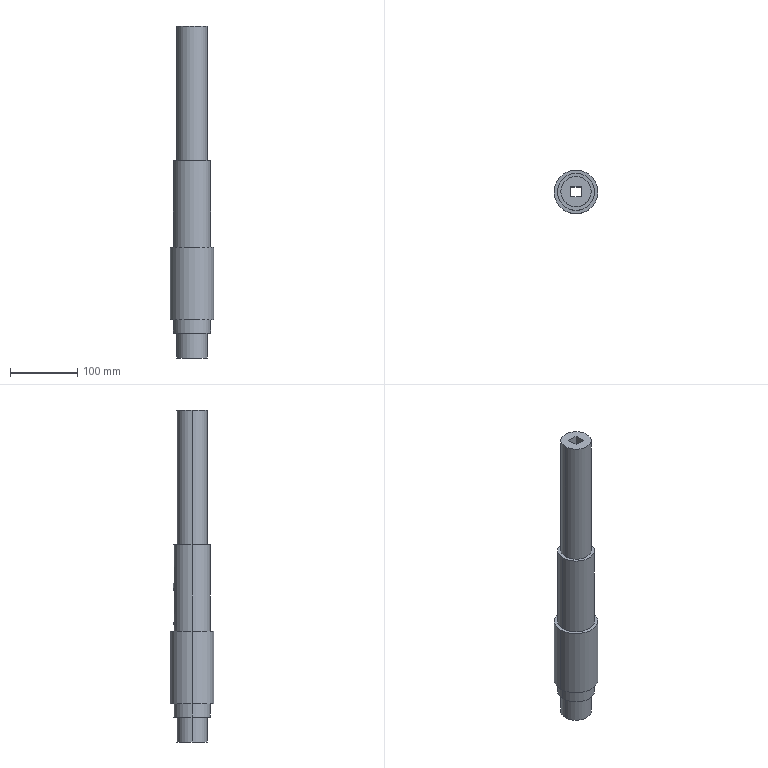Part | SolidWorks | features ICE 2, Chamfer 1, Revolution 1 | 1 solid | 29 faces | box 65 x 65 x 493 mm | volume 970539 mm3 | plane 17 | cylinder 12 | commonest cylinder face diameters 45 x4 55 x4 16 x2 65 x2
STEP:
#1=CARTESIAN_POINT('',(-22.5,0.,293.));
#2=VERTEX_POINT('',#1);
#3=CARTESIAN_POINT('',(22.5,0.,293.));
#4=VERTEX_POINT('',#3);
#5=CARTESIAN_POINT('',(0.,0.,293.));
#6=DIRECTION('',(0.,0.,-1.));
#7=DIRECTION('',(-1.,0.,0.));
#8=AXIS2_PLACEMENT_3D('',#5,#6,#7);
#9=CIRCLE('',#8,22.5);
#10=EDGE_CURVE('',#2,#4,#9,.T.);
#11=ORIENTED_EDGE('',*,*,#10,.T.);
#12=CARTESIAN_POINT('',(22.5,0.,93.));
#13=VERTEX_POINT('',#12);
#14=CARTESIAN_POINT('',(22.5,0.,0.));
#15=DIRECTION('',(0.,0.,-1.));
#16=VECTOR('',#15,1000.);
#17=LINE('',#14,#16);
#18=EDGE_CURVE('',#4,#13,#17,.T.);
#19=ORIENTED_EDGE('',*,*,#18,.T.);
#20=CARTESIAN_POINT('',(-22.5,0.,93.));
#21=VERTEX_POINT('',#20);
#22=CARTESIAN_POINT('',(0.,0.,93.));
#23=DIRECTION('',(0.,0.,-1.));
#24=DIRECTION('',(-1.,0.,0.));
#25=AXIS2_PLACEMENT_3D('',#22,#23,#24);
#26=CIRCLE('',#25,22.5);
#27=EDGE_CURVE('',#21,#13,#26,.T.);
#28=ORIENTED_EDGE('',*,*,#27,.F.);
#29=CARTESIAN_POINT('',(-22.5,0.,0.));
#30=DIRECTION('',(0.,0.,-1.));
#31=VECTOR('',#30,1000.);
#32=LINE('',#29,#31);
#33=EDGE_CURVE('',#2,#21,#32,.T.);
#34=ORIENTED_EDGE('',*,*,#33,.F.);
#35=EDGE_LOOP('',(#11,#19,#28,#34));
#36=FACE_OUTER_BOUND('',#35,.T.);
#37=CARTESIAN_POINT('',(0.,0.,0.));
#38=DIRECTION('',(0.,0.,-1.));
#39=DIRECTION('',(-1.,0.,0.));
#40=AXIS2_PLACEMENT_3D('',#37,#38,#39);
#41=CYLINDRICAL_SURFACE('',#40,22.5);
#42=ADVANCED_FACE('',(#36),#41,.T.);
#43=CARTESIAN_POINT('',(8.,26.311,-17.5));
#44=VERTEX_POINT('',#43);
#45=CARTESIAN_POINT('',(-8.,26.311,-17.5));
#46=VERTEX_POINT('',#45);
#47=CARTESIAN_POINT('',(8.,26.311,-17.5));
#48=CARTESIAN_POINT('',(8.,26.311,-18.032));
#49=CARTESIAN_POINT('',(7.948,26.327,-18.554));
#50=CARTESIAN_POINT('',(7.794,26.372,-19.323));
#51=CARTESIAN_POINT('',(7.73,26.391,-19.577));
#52=CARTESIAN_POINT('',(7.577,26.436,-20.081));
#53=CARTESIAN_POINT('',(7.487,26.461,-20.331));
#54=CARTESIAN_POINT('',(7.185,26.546,-21.056));
#55=CARTESIAN_POINT('',(6.94,26.612,-21.514));
#56=CARTESIAN_POINT('',(6.504,26.72,-22.165));
#57=CARTESIAN_POINT('',(6.347,26.758,-22.376));
#58=CARTESIAN_POINT('',(6.015,26.835,-22.781));
#59=CARTESIAN_POINT('',(5.841,26.873,-22.973));
#60=CARTESIAN_POINT('',(5.29,26.989,-23.523));
#61=CARTESIAN_POINT('',(4.89,27.065,-23.853));
#62=CARTESIAN_POINT('',(4.016,27.209,-24.439));
#63=CARTESIAN_POINT('',(3.556,27.273,-24.685));
#64=CARTESIAN_POINT('',(2.835,27.355,-24.985));
#65=CARTESIAN_POINT('',(2.589,27.379,-25.074));
#66=CARTESIAN_POINT('',(2.087,27.422,-25.227));
#67=CARTESIAN_POINT('',(1.829,27.44,-25.293));
#68=CARTESIAN_POINT('',(1.054,27.485,-25.448));
#69=CARTESIAN_POINT('',(0.5326,27.5,-25.499));
#70=CARTESIAN_POINT('',(-0.5171,27.5,-25.501));
#71=CARTESIAN_POINT('',(-1.05,27.485,-25.448));
#72=CARTESIAN_POINT('',(-2.079,27.426,-25.243));
#73=CARTESIAN_POINT('',(-2.579,27.383,-25.091));
#74=CARTESIAN_POINT('',(-3.308,27.301,-24.789));
#75=CARTESIAN_POINT('',(-3.547,27.271,-24.675));
#76=CARTESIAN_POINT('',(-4.008,27.207,-24.429));
#77=CARTESIAN_POINT('',(-4.231,27.173,-24.295));
#78=CARTESIAN_POINT('',(-4.663,27.103,-24.006));
#79=CARTESIAN_POINT('',(-4.871,27.066,-23.851));
#80=CARTESIAN_POINT('',(-5.275,26.99,-23.52));
#81=CARTESIAN_POINT('',(-5.47,26.951,-23.343));
#82=CARTESIAN_POINT('',(-6.024,26.835,-22.789));
#83=CARTESIAN_POINT('',(-6.354,26.758,-22.389));
#84=CARTESIAN_POINT('',(-6.933,26.613,-21.525));
#85=CARTESIAN_POINT('',(-7.185,26.546,-21.057));
#86=CARTESIAN_POINT('',(-7.586,26.434,-20.094));
#87=CARTESIAN_POINT('',(-7.739,26.389,-19.595));
#88=CARTESIAN_POINT('',(-7.895,26.343,-18.821));
#89=CARTESIAN_POINT('',(-7.934,26.331,-18.558));
#90=CARTESIAN_POINT('',(-7.987,26.315,-18.03));
#91=CARTESIAN_POINT('',(-8.,26.311,-17.766));
#92=CARTESIAN_POINT('',(-8.,26.311,-17.5));
#93=B_SPLINE_CURVE_WITH_KNOTS('',3,(#47,#48,#49,#50,#51,#52,#53,#54,#55,#56,#57,#58,#59,#60,#61,#62,#63,#64,#65,#66,#67,#68,#69,#70,#71,#72,#73,#74,#75,#76,#77,#78,#79,#80,#81,#82,#83,#84,#85,#86,#87,#88,#89,#90,#91,#92),.UNSPECIFIED.,.F.,.F.,(4,2,2,2,2,2,2,2,2,2,2,2,2,2,2,2,2,2,2,2,2,2,4),(0.,0.001571,0.002357,0.003142,0.004714,0.005499,0.006285,0.007856,0.009427,0.01021,0.011,0.01257,0.01414,0.01571,0.0165,0.01728,0.01807,0.01885,0.02043,0.022,0.02357,0.02435,0.02514),.UNSPECIFIED.);
#94=EDGE_CURVE('',#44,#46,#93,.T.);
#95=ORIENTED_EDGE('',*,*,#94,.F.);
#96=CARTESIAN_POINT('',(8.,26.311,19.5));
#97=VERTEX_POINT('',#96);
#98=CARTESIAN_POINT('',(8.,26.311,0.));
#99=DIRECTION('',(0.,0.,-1.));
#100=VECTOR('',#99,1000.);
#101=LINE('',#98,#100);
#102=EDGE_CURVE('',#97,#44,#101,.T.);
#103=ORIENTED_EDGE('',*,*,#102,.F.);
#104=CARTESIAN_POINT('',(-8.,26.311,19.5));
#105=VERTEX_POINT('',#104);
#106=CARTESIAN_POINT('',(-8.,26.311,19.5));
#107=CARTESIAN_POINT('',(-8.,26.311,20.032));
#108=CARTESIAN_POINT('',(-7.948,26.327,20.554));
#109=CARTESIAN_POINT('',(-7.794,26.372,21.323));
#110=CARTESIAN_POINT('',(-7.73,26.391,21.577));
#111=CARTESIAN_POINT('',(-7.577,26.436,22.081));
#112=CARTESIAN_POINT('',(-7.487,26.461,22.331));
#113=CARTESIAN_POINT('',(-7.185,26.546,23.056));
#114=CARTESIAN_POINT('',(-6.94,26.612,23.514));
#115=CARTESIAN_POINT('',(-6.504,26.72,24.165));
#116=CARTESIAN_POINT('',(-6.347,26.758,24.376));
#117=CARTESIAN_POINT('',(-6.015,26.835,24.781));
#118=CARTESIAN_POINT('',(-5.841,26.873,24.973));
#119=CARTESIAN_POINT('',(-5.29,26.989,25.523));
#120=CARTESIAN_POINT('',(-4.89,27.065,25.853));
#121=CARTESIAN_POINT('',(-4.016,27.209,26.439));
#122=CARTESIAN_POINT('',(-3.556,27.273,26.685));
#123=CARTESIAN_POINT('',(-2.835,27.355,26.985));
#124=CARTESIAN_POINT('',(-2.589,27.379,27.074));
#125=CARTESIAN_POINT('',(-2.087,27.422,27.227));
#126=CARTESIAN_POINT('',(-1.829,27.44,27.293));
#127=CARTESIAN_POINT('',(-1.054,27.485,27.448));
#128=CARTESIAN_POINT('',(-0.5326,27.5,27.499));
#129=CARTESIAN_POINT('',(0.5171,27.5,27.501));
#130=CARTESIAN_POINT('',(1.05,27.485,27.448));
#131=CARTESIAN_POINT('',(2.079,27.426,27.243));
#132=CARTESIAN_POINT('',(2.579,27.383,27.091));
#133=CARTESIAN_POINT('',(3.308,27.301,26.789));
#134=CARTESIAN_POINT('',(3.547,27.271,26.675));
#135=CARTESIAN_POINT('',(4.008,27.207,26.429));
#136=CARTESIAN_POINT('',(4.231,27.173,26.295));
#137=CARTESIAN_POINT('',(4.663,27.103,26.006));
#138=CARTESIAN_POINT('',(4.871,27.066,25.851));
#139=CARTESIAN_POINT('',(5.275,26.99,25.52));
#140=CARTESIAN_POINT('',(5.47,26.951,25.343));
#141=CARTESIAN_POINT('',(6.024,26.835,24.789));
#142=CARTESIAN_POINT('',(6.354,26.758,24.389));
#143=CARTESIAN_POINT('',(6.933,26.613,23.525));
#144=CARTESIAN_POINT('',(7.185,26.546,23.057));
#145=CARTESIAN_POINT('',(7.586,26.434,22.094));
#146=CARTESIAN_POINT('',(7.739,26.389,21.595));
#147=CARTESIAN_POINT('',(7.895,26.343,20.821));
#148=CARTESIAN_POINT('',(7.934,26.331,20.558));
#149=CARTESIAN_POINT('',(7.987,26.315,20.03));
#150=CARTESIAN_POINT('',(8.,26.311,19.766));
#151=CARTESIAN_POINT('',(8.,26.311,19.5));
#152=B_SPLINE_CURVE_WITH_KNOTS('',3,(#106,#107,#108,#109,#110,#111,#112,#113,#114,#115,#116,#117,#118,#119,#120,#121,#122,#123,#124,#125,#126,#127,#128,#129,#130,#131,#132,#133,#134,#135,#136,#137,#138,#139,#140,#141,#142,#143,#144,#145,#146,#147,#148,#149,#150,#151),.UNSPECIFIED.,.F.,.F.,(4,2,2,2,2,2,2,2,2,2,2,2,2,2,2,2,2,2,2,2,2,2,4),(0.,0.001571,0.002357,0.003142,0.004714,0.005499,0.006285,0.007856,0.009427,0.01021,0.011,0.01257,0.01414,0.01571,0.0165,0.01728,0.01807,0.01885,0.02043,0.022,0.02357,0.02435,0.02514),.UNSPECIFIED.);
#153=EDGE_CURVE('',#105,#97,#152,.T.);
#154=ORIENTED_EDGE('',*,*,#153,.F.);
#155=CARTESIAN_POINT('',(-8.,26.311,0.));
#156=DIRECTION('',(0.,0.,1.));
#157=VECTOR('',#156,1000.);
#158=LINE('',#155,#157);
#159=EDGE_CURVE('',#46,#105,#158,.T.);
#160=ORIENTED_EDGE('',*,*,#159,.F.);
#161=EDGE_LOOP('',(#95,#103,#154,#160));
#162=FACE_BOUND('',#161,.T.);
#163=CARTESIAN_POINT('',(-27.5,0.,93.));
#164=VERTEX_POINT('',#163);
#165=CARTESIAN_POINT('',(27.5,0.,93.));
#166=VERTEX_POINT('',#165);
#167=CARTESIAN_POINT('',(0.,0.,93.));
#168=DIRECTION('',(0.,0.,-1.));
#169=DIRECTION('',(-1.,0.,0.));
#170=AXIS2_PLACEMENT_3D('',#167,#168,#169);
#171=CIRCLE('',#170,27.5);
#172=EDGE_CURVE('',#164,#166,#171,.T.);
#173=ORIENTED_EDGE('',*,*,#172,.T.);
#174=CARTESIAN_POINT('',(27.5,0.,-35.5));
#175=VERTEX_POINT('',#174);
#176=CARTESIAN_POINT('',(27.5,0.,0.));
#177=DIRECTION('',(0.,0.,-1.));
#178=VECTOR('',#177,1000.);
#179=LINE('',#176,#178);
#180=EDGE_CURVE('',#166,#175,#179,.T.);
#181=ORIENTED_EDGE('',*,*,#180,.T.);
#182=CARTESIAN_POINT('',(-27.5,0.,-35.5));
#183=VERTEX_POINT('',#182);
#184=CARTESIAN_POINT('',(0.,0.,-35.5));
#185=DIRECTION('',(0.,0.,-1.));
#186=DIRECTION('',(-1.,0.,0.));
#187=AXIS2_PLACEMENT_3D('',#184,#185,#186);
#188=CIRCLE('',#187,27.5);
#189=EDGE_CURVE('',#183,#175,#188,.T.);
#190=ORIENTED_EDGE('',*,*,#189,.F.);
#191=CARTESIAN_POINT('',(-27.5,0.,0.));
#192=DIRECTION('',(0.,0.,-1.));
#193=VECTOR('',#192,1000.);
#194=LINE('',#191,#193);
#195=EDGE_CURVE('',#164,#183,#194,.T.);
#196=ORIENTED_EDGE('',*,*,#195,.F.);
#197=EDGE_LOOP('',(#173,#181,#190,#196));
#198=FACE_OUTER_BOUND('',#197,.T.);
#199=CARTESIAN_POINT('',(0.,0.,0.));
#200=DIRECTION('',(0.,0.,-1.));
#201=DIRECTION('',(-1.,0.,0.));
#202=AXIS2_PLACEMENT_3D('',#199,#200,#201);
#203=CYLINDRICAL_SURFACE('',#202,27.5);
#204=ADVANCED_FACE('',(#162,#198),#203,.T.);
#205=CARTESIAN_POINT('',(-32.5,0.,-35.5));
#206=VERTEX_POINT('',#205);
#207=CARTESIAN_POINT('',(32.5,0.,-35.5));
#208=VERTEX_POINT('',#207);
#209=CARTESIAN_POINT('',(0.,0.,-35.5));
#210=DIRECTION('',(0.,0.,-1.));
#211=DIRECTION('',(-1.,0.,0.));
#212=AXIS2_PLACEMENT_3D('',#209,#210,#211);
#213=CIRCLE('',#212,32.5);
#214=EDGE_CURVE('',#206,#208,#213,.T.);
#215=ORIENTED_EDGE('',*,*,#214,.T.);
#216=CARTESIAN_POINT('',(32.5,0.,-143.));
#217=VERTEX_POINT('',#216);
#218=CARTESIAN_POINT('',(32.5,0.,0.));
#219=DIRECTION('',(0.,0.,-1.));
#220=VECTOR('',#219,1000.);
#221=LINE('',#218,#220);
#222=EDGE_CURVE('',#208,#217,#221,.T.);
#223=ORIENTED_EDGE('',*,*,#222,.T.);
#224=CARTESIAN_POINT('',(-32.5,0.,-143.));
#225=VERTEX_POINT('',#224);
#226=CARTESIAN_POINT('',(0.,0.,-143.));
#227=DIRECTION('',(0.,0.,-1.));
#228=DIRECTION('',(-1.,0.,0.));
#229=AXIS2_PLACEMENT_3D('',#226,#227,#228);
#230=CIRCLE('',#229,32.5);
#231=EDGE_CURVE('',#225,#217,#230,.T.);
#232=ORIENTED_EDGE('',*,*,#231,.F.);
#233=CARTESIAN_POINT('',(-32.5,0.,0.));
#234=DIRECTION('',(0.,0.,-1.));
#235=VECTOR('',#234,1000.);
#236=LINE('',#233,#235);
#237=EDGE_CURVE('',#206,#225,#236,.T.);
#238=ORIENTED_EDGE('',*,*,#237,.F.);
#239=EDGE_LOOP('',(#215,#223,#232,#238));
#240=FACE_OUTER_BOUND('',#239,.T.);
#241=CARTESIAN_POINT('',(0.,0.,0.));
#242=DIRECTION('',(0.,0.,-1.));
#243=DIRECTION('',(-1.,0.,0.));
#244=AXIS2_PLACEMENT_3D('',#241,#242,#243);
#245=CYLINDRICAL_SURFACE('',#244,32.5);
#246=ADVANCED_FACE('',(#240),#245,.T.);
#247=CARTESIAN_POINT('',(-27.5,0.,-143.));
#248=VERTEX_POINT('',#247);
#249=CARTESIAN_POINT('',(27.5,0.,-143.));
#250=VERTEX_POINT('',#249);
#251=CARTESIAN_POINT('',(0.,0.,-143.));
#252=DIRECTION('',(0.,0.,-1.));
#253=DIRECTION('',(-1.,0.,0.));
#254=AXIS2_PLACEMENT_3D('',#251,#252,#253);
#255=CIRCLE('',#254,27.5);
#256=EDGE_CURVE('',#248,#250,#255,.T.);
#257=ORIENTED_EDGE('',*,*,#256,.T.);
#258=CARTESIAN_POINT('',(27.5,0.,-163.));
#259=VERTEX_POINT('',#258);
#260=CARTESIAN_POINT('',(27.5,0.,0.));
#261=DIRECTION('',(0.,0.,-1.));
#262=VECTOR('',#261,1000.);
#263=LINE('',#260,#262);
#264=EDGE_CURVE('',#250,#259,#263,.T.);
#265=ORIENTED_EDGE('',*,*,#264,.T.);
#266=CARTESIAN_POINT('',(-27.5,0.,-163.));
#267=VERTEX_POINT('',#266);
#268=CARTESIAN_POINT('',(0.,0.,-163.));
#269=DIRECTION('',(0.,0.,-1.));
#270=DIRECTION('',(-1.,0.,0.));
#271=AXIS2_PLACEMENT_3D('',#268,#269,#270);
#272=CIRCLE('',#271,27.5);
#273=EDGE_CURVE('',#267,#259,#272,.T.);
#274=ORIENTED_EDGE('',*,*,#273,.F.);
#275=CARTESIAN_POINT('',(-27.5,0.,0.));
#276=DIRECTION('',(0.,0.,-1.));
#277=VECTOR('',#276,1000.);
#278=LINE('',#275,#277);
#279=EDGE_CURVE('',#248,#267,#278,.T.);
#280=ORIENTED_EDGE('',*,*,#279,.F.);
#281=EDGE_LOOP('',(#257,#265,#274,#280));
#282=FACE_OUTER_BOUND('',#281,.T.);
#283=CARTESIAN_POINT('',(0.,0.,0.));
#284=DIRECTION('',(0.,0.,-1.));
#285=DIRECTION('',(-1.,0.,0.));
#286=AXIS2_PLACEMENT_3D('',#283,#284,#285);
#287=CYLINDRICAL_SURFACE('',#286,27.5);
#288=ADVANCED_FACE('',(#282),#287,.T.);
#289=CARTESIAN_POINT('',(-22.5,0.,-163.));
#290=VERTEX_POINT('',#289);
#291=CARTESIAN_POINT('',(22.5,0.,-163.));
#292=VERTEX_POINT('',#291);
#293=CARTESIAN_POINT('',(0.,0.,-163.));
#294=DIRECTION('',(0.,0.,-1.));
#295=DIRECTION('',(-1.,0.,0.));
#296=AXIS2_PLACEMENT_3D('',#293,#294,#295);
#297=CIRCLE('',#296,22.5);
#298=EDGE_CURVE('',#290,#292,#297,.T.);
#299=ORIENTED_EDGE('',*,*,#298,.T.);
#300=CARTESIAN_POINT('',(22.5,0.,-200.));
#301=VERTEX_POINT('',#300);
#302=CARTESIAN_POINT('',(22.5,0.,0.));
#303=DIRECTION('',(0.,0.,-1.));
#304=VECTOR('',#303,1000.);
#305=LINE('',#302,#304);
#306=EDGE_CURVE('',#292,#301,#305,.T.);
#307=ORIENTED_EDGE('',*,*,#306,.T.);
#308=CARTESIAN_POINT('',(-22.5,0.,-200.));
#309=VERTEX_POINT('',#308);
#310=CARTESIAN_POINT('',(0.,0.,-200.));
#311=DIRECTION('',(0.,0.,-1.));
#312=DIRECTION('',(-1.,0.,0.));
#313=AXIS2_PLACEMENT_3D('',#310,#311,#312);
#314=CIRCLE('',#313,22.5);
#315=EDGE_CURVE('',#309,#301,#314,.T.);
#316=ORIENTED_EDGE('',*,*,#315,.F.);
#317=CARTESIAN_POINT('',(-22.5,0.,0.));
#318=DIRECTION('',(0.,0.,-1.));
#319=VECTOR('',#318,1000.);
#320=LINE('',#317,#319);
#321=EDGE_CURVE('',#290,#309,#320,.T.);
#322=ORIENTED_EDGE('',*,*,#321,.F.);
#323=EDGE_LOOP('',(#299,#307,#316,#322));
#324=FACE_OUTER_BOUND('',#323,.T.);
#325=CARTESIAN_POINT('',(0.,0.,0.));
#326=DIRECTION('',(0.,0.,-1.));
#327=DIRECTION('',(-1.,0.,0.));
#328=AXIS2_PLACEMENT_3D('',#325,#326,#327);
#329=CYLINDRICAL_SURFACE('',#328,22.5);
#330=ADVANCED_FACE('',(#324),#329,.T.);
#331=CARTESIAN_POINT('',(-10.5,-10.5,-200.));
#332=VERTEX_POINT('',#331);
#333=CARTESIAN_POINT('',(10.5,-10.5,-200.));
#334=VERTEX_POINT('',#333);
#335=CARTESIAN_POINT('',(7.5,-10.5,-200.));
#336=DIRECTION('',(1.,0.,0.));
#337=VECTOR('',#336,1000.);
#338=LINE('',#335,#337);
#339=EDGE_CURVE('',#332,#334,#338,.T.);
#340=ORIENTED_EDGE('',*,*,#339,.T.);
#341=CARTESIAN_POINT('',(10.5,10.5,-200.));
#342=VERTEX_POINT('',#341);
#343=CARTESIAN_POINT('',(10.5,7.5,-200.));
#344=DIRECTION('',(0.,1.,0.));
#345=VECTOR('',#344,1000.);
#346=LINE('',#343,#345);
#347=EDGE_CURVE('',#334,#342,#346,.T.);
#348=ORIENTED_EDGE('',*,*,#347,.T.);
#349=CARTESIAN_POINT('',(-10.5,10.5,-200.));
#350=VERTEX_POINT('',#349);
#351=CARTESIAN_POINT('',(-7.5,10.5,-200.));
#352=DIRECTION('',(-1.,0.,0.));
#353=VECTOR('',#352,1000.);
#354=LINE('',#351,#353);
#355=EDGE_CURVE('',#342,#350,#354,.T.);
#356=ORIENTED_EDGE('',*,*,#355,.T.);
#357=CARTESIAN_POINT('',(-10.5,-7.5,-200.));
#358=DIRECTION('',(0.,-1.,0.));
#359=VECTOR('',#358,1000.);
#360=LINE('',#357,#359);
#361=EDGE_CURVE('',#350,#332,#360,.T.);
#362=ORIENTED_EDGE('',*,*,#361,.T.);
#363=EDGE_LOOP('',(#340,#348,#356,#362));
#364=FACE_BOUND('',#363,.T.);
#365=ORIENTED_EDGE('',*,*,#315,.T.);
#366=CARTESIAN_POINT('',(0.,0.,-200.));
#367=DIRECTION('',(0.,0.,-1.));
#368=DIRECTION('',(-1.,0.,0.));
#369=AXIS2_PLACEMENT_3D('',#366,#367,#368);
#370=CIRCLE('',#369,22.5);
#371=EDGE_CURVE('',#301,#309,#370,.T.);
#372=ORIENTED_EDGE('',*,*,#371,.T.);
#373=EDGE_LOOP('',(#365,#372));
#374=FACE_OUTER_BOUND('',#373,.T.);
#375=CARTESIAN_POINT('',(0.,0.,-200.));
#376=DIRECTION('',(0.,0.,-1.));
#377=DIRECTION('',(-1.,0.,0.));
#378=AXIS2_PLACEMENT_3D('',#375,#376,#377);
#379=PLANE('',#378);
#380=ADVANCED_FACE('',(#364,#374),#379,.T.);
#381=ORIENTED_EDGE('',*,*,#306,.F.);
#382=CARTESIAN_POINT('',(0.,0.,-163.));
#383=DIRECTION('',(0.,0.,-1.));
#384=DIRECTION('',(-1.,0.,0.));
#385=AXIS2_PLACEMENT_3D('',#382,#383,#384);
#386=CIRCLE('',#385,22.5);
#387=EDGE_CURVE('',#292,#290,#386,.T.);
#388=ORIENTED_EDGE('',*,*,#387,.T.);
#389=ORIENTED_EDGE('',*,*,#321,.T.);
#390=ORIENTED_EDGE('',*,*,#371,.F.);
#391=EDGE_LOOP('',(#381,#388,#389,#390));
#392=FACE_OUTER_BOUND('',#391,.T.);
#393=CARTESIAN_POINT('',(0.,0.,0.));
#394=DIRECTION('',(0.,0.,-1.));
#395=DIRECTION('',(-1.,0.,0.));
#396=AXIS2_PLACEMENT_3D('',#393,#394,#395);
#397=CYLINDRICAL_SURFACE('',#396,22.5);
#398=ADVANCED_FACE('',(#392),#397,.T.);
#399=ORIENTED_EDGE('',*,*,#273,.T.);
#400=CARTESIAN_POINT('',(0.,0.,-163.));
#401=DIRECTION('',(0.,0.,-1.));
#402=DIRECTION('',(-1.,0.,0.));
#403=AXIS2_PLACEMENT_3D('',#400,#401,#402);
#404=CIRCLE('',#403,27.5);
#405=EDGE_CURVE('',#259,#267,#404,.T.);
#406=ORIENTED_EDGE('',*,*,#405,.T.);
#407=EDGE_LOOP('',(#399,#406));
#408=FACE_OUTER_BOUND('',#407,.T.);
#409=ORIENTED_EDGE('',*,*,#298,.F.);
#410=ORIENTED_EDGE('',*,*,#387,.F.);
#411=EDGE_LOOP('',(#409,#410));
#412=FACE_BOUND('',#411,.T.);
#413=CARTESIAN_POINT('',(-22.5,0.,-163.));
#414=DIRECTION('',(0.,0.,-1.));
#415=DIRECTION('',(-1.,0.,0.));
#416=AXIS2_PLACEMENT_3D('',#413,#414,#415);
#417=PLANE('',#416);
#418=ADVANCED_FACE('',(#408,#412),#417,.T.);
#419=ORIENTED_EDGE('',*,*,#264,.F.);
#420=CARTESIAN_POINT('',(0.,0.,-143.));
#421=DIRECTION('',(0.,0.,-1.));
#422=DIRECTION('',(-1.,0.,0.));
#423=AXIS2_PLACEMENT_3D('',#420,#421,#422);
#424=CIRCLE('',#423,27.5);
#425=EDGE_CURVE('',#250,#248,#424,.T.);
#426=ORIENTED_EDGE('',*,*,#425,.T.);
#427=ORIENTED_EDGE('',*,*,#279,.T.);
#428=ORIENTED_EDGE('',*,*,#405,.F.);
#429=EDGE_LOOP('',(#419,#426,#427,#428));
#430=FACE_OUTER_BOUND('',#429,.T.);
#431=CARTESIAN_POINT('',(0.,0.,0.));
#432=DIRECTION('',(0.,0.,-1.));
#433=DIRECTION('',(-1.,0.,0.));
#434=AXIS2_PLACEMENT_3D('',#431,#432,#433);
#435=CYLINDRICAL_SURFACE('',#434,27.5);
#436=ADVANCED_FACE('',(#430),#435,.T.);
#437=ORIENTED_EDGE('',*,*,#231,.T.);
#438=CARTESIAN_POINT('',(0.,0.,-143.));
#439=DIRECTION('',(0.,0.,-1.));
#440=DIRECTION('',(-1.,0.,0.));
#441=AXIS2_PLACEMENT_3D('',#438,#439,#440);
#442=CIRCLE('',#441,32.5);
#443=EDGE_CURVE('',#217,#225,#442,.T.);
#444=ORIENTED_EDGE('',*,*,#443,.T.);
#445=EDGE_LOOP('',(#437,#444));
#446=FACE_OUTER_BOUND('',#445,.T.);
#447=ORIENTED_EDGE('',*,*,#256,.F.);
#448=ORIENTED_EDGE('',*,*,#425,.F.);
#449=EDGE_LOOP('',(#447,#448));
#450=FACE_BOUND('',#449,.T.);
#451=CARTESIAN_POINT('',(-32.5,0.,-143.));
#452=DIRECTION('',(0.,0.,-1.));
#453=DIRECTION('',(-1.,0.,0.));
#454=AXIS2_PLACEMENT_3D('',#451,#452,#453);
#455=PLANE('',#454);
#456=ADVANCED_FACE('',(#446,#450),#455,.T.);
#457=ORIENTED_EDGE('',*,*,#222,.F.);
#458=CARTESIAN_POINT('',(0.,0.,-35.5));
#459=DIRECTION('',(0.,0.,-1.));
#460=DIRECTION('',(-1.,0.,0.));
#461=AXIS2_PLACEMENT_3D('',#458,#459,#460);
#462=CIRCLE('',#461,32.5);
#463=EDGE_CURVE('',#208,#206,#462,.T.);
#464=ORIENTED_EDGE('',*,*,#463,.T.);
#465=ORIENTED_EDGE('',*,*,#237,.T.);
#466=ORIENTED_EDGE('',*,*,#443,.F.);
#467=EDGE_LOOP('',(#457,#464,#465,#466));
#468=FACE_OUTER_BOUND('',#467,.T.);
#469=CARTESIAN_POINT('',(0.,0.,0.));
#470=DIRECTION('',(0.,0.,-1.));
#471=DIRECTION('',(-1.,0.,0.));
#472=AXIS2_PLACEMENT_3D('',#469,#470,#471);
#473=CYLINDRICAL_SURFACE('',#472,32.5);
#474=ADVANCED_FACE('',(#468),#473,.T.);
#475=ORIENTED_EDGE('',*,*,#189,.T.);
#476=CARTESIAN_POINT('',(0.,0.,-35.5));
#477=DIRECTION('',(0.,0.,-1.));
#478=DIRECTION('',(-1.,0.,0.));
#479=AXIS2_PLACEMENT_3D('',#476,#477,#478);
#480=CIRCLE('',#479,27.5);
#481=EDGE_CURVE('',#175,#183,#480,.T.);
#482=ORIENTED_EDGE('',*,*,#481,.T.);
#483=EDGE_LOOP('',(#475,#482));
#484=FACE_BOUND('',#483,.T.);
#485=ORIENTED_EDGE('',*,*,#214,.F.);
#486=ORIENTED_EDGE('',*,*,#463,.F.);
#487=EDGE_LOOP('',(#485,#486));
#488=FACE_OUTER_BOUND('',#487,.T.);
#489=CARTESIAN_POINT('',(-27.5,0.,-35.5));
#490=DIRECTION('',(0.,0.,1.));
#491=DIRECTION('',(1.,0.,0.));
#492=AXIS2_PLACEMENT_3D('',#489,#490,#491);
#493=PLANE('',#492);
#494=ADVANCED_FACE('',(#484,#488),#493,.T.);
#495=ORIENTED_EDGE('',*,*,#180,.F.);
#496=CARTESIAN_POINT('',(0.,0.,93.));
#497=DIRECTION('',(0.,0.,-1.));
#498=DIRECTION('',(-1.,0.,0.));
#499=AXIS2_PLACEMENT_3D('',#496,#497,#498);
#500=CIRCLE('',#499,27.5);
#501=EDGE_CURVE('',#166,#164,#500,.T.);
#502=ORIENTED_EDGE('',*,*,#501,.T.);
#503=ORIENTED_EDGE('',*,*,#195,.T.);
#504=ORIENTED_EDGE('',*,*,#481,.F.);
#505=EDGE_LOOP('',(#495,#502,#503,#504));
#506=FACE_OUTER_BOUND('',#505,.T.);
#507=CARTESIAN_POINT('',(0.,0.,0.));
#508=DIRECTION('',(0.,0.,-1.));
#509=DIRECTION('',(-1.,0.,0.));
#510=AXIS2_PLACEMENT_3D('',#507,#508,#509);
#511=CYLINDRICAL_SURFACE('',#510,27.5);
#512=ADVANCED_FACE('',(#506),#511,.T.);
#513=ORIENTED_EDGE('',*,*,#27,.T.);
#514=CARTESIAN_POINT('',(0.,0.,93.));
#515=DIRECTION('',(0.,0.,-1.));
#516=DIRECTION('',(-1.,0.,0.));
#517=AXIS2_PLACEMENT_3D('',#514,#515,#516);
#518=CIRCLE('',#517,22.5);
#519=EDGE_CURVE('',#13,#21,#518,.T.);
#520=ORIENTED_EDGE('',*,*,#519,.T.);
#521=EDGE_LOOP('',(#513,#520));
#522=FACE_BOUND('',#521,.T.);
#523=ORIENTED_EDGE('',*,*,#172,.F.);
#524=ORIENTED_EDGE('',*,*,#501,.F.);
#525=EDGE_LOOP('',(#523,#524));
#526=FACE_OUTER_BOUND('',#525,.T.);
#527=CARTESIAN_POINT('',(-27.5,0.,93.));
#528=DIRECTION('',(0.,0.,1.));
#529=DIRECTION('',(1.,0.,0.));
#530=AXIS2_PLACEMENT_3D('',#527,#528,#529);
#531=PLANE('',#530);
#532=ADVANCED_FACE('',(#522,#526),#531,.T.);
#533=ORIENTED_EDGE('',*,*,#18,.F.);
#534=CARTESIAN_POINT('',(0.,0.,293.));
#535=DIRECTION('',(0.,0.,-1.));
#536=DIRECTION('',(-1.,0.,0.));
#537=AXIS2_PLACEMENT_3D('',#534,#535,#536);
#538=CIRCLE('',#537,22.5);
#539=EDGE_CURVE('',#4,#2,#538,.T.);
#540=ORIENTED_EDGE('',*,*,#539,.T.);
#541=ORIENTED_EDGE('',*,*,#33,.T.);
#542=ORIENTED_EDGE('',*,*,#519,.F.);
#543=EDGE_LOOP('',(#533,#540,#541,#542));
#544=FACE_OUTER_BOUND('',#543,.T.);
#545=CARTESIAN_POINT('',(0.,0.,0.));
#546=DIRECTION('',(0.,0.,-1.));
#547=DIRECTION('',(-1.,0.,0.));
#548=AXIS2_PLACEMENT_3D('',#545,#546,#547);
#549=CYLINDRICAL_SURFACE('',#548,22.5);
#550=ADVANCED_FACE('',(#544),#549,.T.);
#551=CARTESIAN_POINT('',(7.5,7.5,293.));
#552=VERTEX_POINT('',#551);
#553=CARTESIAN_POINT('',(7.5,-7.5,293.));
#554=VERTEX_POINT('',#553);
#555=CARTESIAN_POINT('',(7.5,7.5,293.));
#556=DIRECTION('',(0.,-1.,0.));
#557=VECTOR('',#556,1000.);
#558=LINE('',#555,#557);
#559=EDGE_CURVE('',#552,#554,#558,.T.);
#560=ORIENTED_EDGE('',*,*,#559,.T.);
#561=CARTESIAN_POINT('',(-7.5,-7.5,293.));
#562=VERTEX_POINT('',#561);
#563=CARTESIAN_POINT('',(-7.5,-7.5,293.));
#564=DIRECTION('',(-1.,0.,0.));
#565=VECTOR('',#564,1000.);
#566=LINE('',#563,#565);
#567=EDGE_CURVE('',#554,#562,#566,.T.);
#568=ORIENTED_EDGE('',*,*,#567,.T.);
#569=CARTESIAN_POINT('',(-7.5,7.5,293.));
#570=VERTEX_POINT('',#569);
#571=CARTESIAN_POINT('',(-7.5,7.5,293.));
#572=DIRECTION('',(0.,1.,0.));
#573=VECTOR('',#572,1000.);
#574=LINE('',#571,#573);
#575=EDGE_CURVE('',#562,#570,#574,.T.);
#576=ORIENTED_EDGE('',*,*,#575,.T.);
#577=CARTESIAN_POINT('',(-7.5,7.5,293.));
#578=DIRECTION('',(1.,0.,0.));
#579=VECTOR('',#578,1000.);
#580=LINE('',#577,#579);
#581=EDGE_CURVE('',#570,#552,#580,.T.);
#582=ORIENTED_EDGE('',*,*,#581,.T.);
#583=EDGE_LOOP('',(#560,#568,#576,#582));
#584=FACE_BOUND('',#583,.T.);
#585=ORIENTED_EDGE('',*,*,#10,.F.);
#586=ORIENTED_EDGE('',*,*,#539,.F.);
#587=EDGE_LOOP('',(#585,#586));
#588=FACE_OUTER_BOUND('',#587,.T.);
#589=CARTESIAN_POINT('',(-22.5,0.,293.));
#590=DIRECTION('',(0.,0.,1.));
#591=DIRECTION('',(1.,0.,0.));
#592=AXIS2_PLACEMENT_3D('',#589,#590,#591);
#593=PLANE('',#592);
#594=ADVANCED_FACE('',(#584,#588),#593,.T.);
#595=CARTESIAN_POINT('',(7.5,7.5,-194.804));
#596=VERTEX_POINT('',#595);
#597=CARTESIAN_POINT('',(7.5,7.5,293.));
#598=DIRECTION('',(0.,0.,-1.));
#599=VECTOR('',#598,1000.);
#600=LINE('',#597,#599);
#601=EDGE_CURVE('',#552,#596,#600,.T.);
#602=ORIENTED_EDGE('',*,*,#601,.T.);
#603=CARTESIAN_POINT('',(7.5,-7.5,-194.804));
#604=VERTEX_POINT('',#603);
#605=CARTESIAN_POINT('',(7.5,-7.5,-194.804));
#606=DIRECTION('',(0.,-1.,0.));
#607=VECTOR('',#606,1000.);
#608=LINE('',#605,#607);
#609=EDGE_CURVE('',#596,#604,#608,.T.);
#610=ORIENTED_EDGE('',*,*,#609,.T.);
#611=CARTESIAN_POINT('',(7.5,-7.5,293.));
#612=DIRECTION('',(0.,0.,-1.));
#613=VECTOR('',#612,1000.);
#614=LINE('',#611,#613);
#615=EDGE_CURVE('',#554,#604,#614,.T.);
#616=ORIENTED_EDGE('',*,*,#615,.F.);
#617=ORIENTED_EDGE('',*,*,#559,.F.);
#618=EDGE_LOOP('',(#602,#610,#616,#617));
#619=FACE_OUTER_BOUND('',#618,.T.);
#620=CARTESIAN_POINT('',(7.5,7.5,293.));
#621=DIRECTION('',(1.,0.,0.));
#622=DIRECTION('',(0.,1.,0.));
#623=AXIS2_PLACEMENT_3D('',#620,#621,#622);
#624=PLANE('',#623);
#625=ADVANCED_FACE('',(#619),#624,.F.);
#626=CARTESIAN_POINT('',(-7.5,7.5,-194.804));
#627=VERTEX_POINT('',#626);
#628=CARTESIAN_POINT('',(-7.5,7.5,293.));
#629=DIRECTION('',(0.,0.,-1.));
#630=VECTOR('',#629,1000.);
#631=LINE('',#628,#630);
#632=EDGE_CURVE('',#570,#627,#631,.T.);
#633=ORIENTED_EDGE('',*,*,#632,.T.);
#634=CARTESIAN_POINT('',(7.5,7.5,-194.804));
#635=DIRECTION('',(1.,0.,0.));
#636=VECTOR('',#635,1000.);
#637=LINE('',#634,#636);
#638=EDGE_CURVE('',#627,#596,#637,.T.);
#639=ORIENTED_EDGE('',*,*,#638,.T.);
#640=ORIENTED_EDGE('',*,*,#601,.F.);
#641=ORIENTED_EDGE('',*,*,#581,.F.);
#642=EDGE_LOOP('',(#633,#639,#640,#641));
#643=FACE_OUTER_BOUND('',#642,.T.);
#644=CARTESIAN_POINT('',(-7.5,7.5,293.));
#645=DIRECTION('',(0.,1.,0.));
#646=DIRECTION('',(-1.,0.,0.));
#647=AXIS2_PLACEMENT_3D('',#644,#645,#646);
#648=PLANE('',#647);
#649=ADVANCED_FACE('',(#643),#648,.F.);
#650=CARTESIAN_POINT('',(-7.5,-7.5,-194.804));
#651=VERTEX_POINT('',#650);
#652=CARTESIAN_POINT('',(-7.5,-7.5,293.));
#653=DIRECTION('',(0.,0.,-1.));
#654=VECTOR('',#653,1000.);
#655=LINE('',#652,#654);
#656=EDGE_CURVE('',#562,#651,#655,.T.);
#657=ORIENTED_EDGE('',*,*,#656,.T.);
#658=CARTESIAN_POINT('',(-7.5,7.5,-194.804));
#659=DIRECTION('',(0.,1.,0.));
#660=VECTOR('',#659,1000.);
#661=LINE('',#658,#660);
#662=EDGE_CURVE('',#651,#627,#661,.T.);
#663=ORIENTED_EDGE('',*,*,#662,.T.);
#664=ORIENTED_EDGE('',*,*,#632,.F.);
#665=ORIENTED_EDGE('',*,*,#575,.F.);
#666=EDGE_LOOP('',(#657,#663,#664,#665));
#667=FACE_OUTER_BOUND('',#666,.T.);
#668=CARTESIAN_POINT('',(-7.5,7.5,293.));
#669=DIRECTION('',(-1.,0.,0.));
#670=DIRECTION('',(0.,-1.,0.));
#671=AXIS2_PLACEMENT_3D('',#668,#669,#670);
#672=PLANE('',#671);
#673=ADVANCED_FACE('',(#667),#672,.F.);
#674=ORIENTED_EDGE('',*,*,#615,.T.);
#675=CARTESIAN_POINT('',(-7.5,-7.5,-194.804));
#676=DIRECTION('',(-1.,0.,0.));
#677=VECTOR('',#676,1000.);
#678=LINE('',#675,#677);
#679=EDGE_CURVE('',#604,#651,#678,.T.);
#680=ORIENTED_EDGE('',*,*,#679,.T.);
#681=ORIENTED_EDGE('',*,*,#656,.F.);
#682=ORIENTED_EDGE('',*,*,#567,.F.);
#683=EDGE_LOOP('',(#674,#680,#681,#682));
#684=FACE_OUTER_BOUND('',#683,.T.);
#685=CARTESIAN_POINT('',(-7.5,-7.5,293.));
#686=DIRECTION('',(0.,-1.,0.));
#687=DIRECTION('',(1.,0.,0.));
#688=AXIS2_PLACEMENT_3D('',#685,#686,#687);
#689=PLANE('',#688);
#690=ADVANCED_FACE('',(#684),#689,.F.);
#691=CARTESIAN_POINT('',(-4.5,-4.5,-189.608));
#692=DIRECTION('',(0.4472,0.4472,0.7746));
#693=VECTOR('',#692,1000.);
#694=LINE('',#691,#693);
#695=EDGE_CURVE('',#332,#651,#694,.T.);
#696=ORIENTED_EDGE('',*,*,#695,.F.);
#697=ORIENTED_EDGE('',*,*,#361,.F.);
#698=CARTESIAN_POINT('',(-7.5,7.5,-194.804));
#699=DIRECTION('',(-0.4472,0.4472,-0.7746));
#700=VECTOR('',#699,1000.);
#701=LINE('',#698,#700);
#702=EDGE_CURVE('',#627,#350,#701,.T.);
#703=ORIENTED_EDGE('',*,*,#702,.F.);
#704=ORIENTED_EDGE('',*,*,#662,.F.);
#705=EDGE_LOOP('',(#696,#697,#703,#704));
#706=FACE_OUTER_BOUND('',#705,.T.);
#707=CARTESIAN_POINT('',(-7.5,7.5,-194.804));
#708=DIRECTION('',(0.866,0.,-0.5));
#709=DIRECTION('',(0.,-1.,0.));
#710=AXIS2_PLACEMENT_3D('',#707,#708,#709);
#711=PLANE('',#710);
#712=ADVANCED_FACE('',(#706),#711,.T.);
#713=ORIENTED_EDGE('',*,*,#702,.T.);
#714=ORIENTED_EDGE('',*,*,#355,.F.);
#715=CARTESIAN_POINT('',(7.5,7.5,-194.804));
#716=DIRECTION('',(0.4472,0.4472,-0.7746));
#717=VECTOR('',#716,1000.);
#718=LINE('',#715,#717);
#719=EDGE_CURVE('',#596,#342,#718,.T.);
#720=ORIENTED_EDGE('',*,*,#719,.F.);
#721=ORIENTED_EDGE('',*,*,#638,.F.);
#722=EDGE_LOOP('',(#713,#714,#720,#721));
#723=FACE_OUTER_BOUND('',#722,.T.);
#724=CARTESIAN_POINT('',(-7.5,7.5,-194.804));
#725=DIRECTION('',(0.,-0.866,-0.5));
#726=DIRECTION('',(-1.,0.,0.));
#727=AXIS2_PLACEMENT_3D('',#724,#725,#726);
#728=PLANE('',#727);
#729=ADVANCED_FACE('',(#723),#728,.T.);
#730=ORIENTED_EDGE('',*,*,#695,.T.);
#731=ORIENTED_EDGE('',*,*,#679,.F.);
#732=CARTESIAN_POINT('',(4.5,-4.5,-189.608));
#733=DIRECTION('',(-0.4472,0.4472,0.7746));
#734=VECTOR('',#733,1000.);
#735=LINE('',#732,#734);
#736=EDGE_CURVE('',#334,#604,#735,.T.);
#737=ORIENTED_EDGE('',*,*,#736,.F.);
#738=ORIENTED_EDGE('',*,*,#339,.F.);
#739=EDGE_LOOP('',(#730,#731,#737,#738));
#740=FACE_OUTER_BOUND('',#739,.T.);
#741=CARTESIAN_POINT('',(-7.5,-7.5,-194.804));
#742=DIRECTION('',(0.,0.866,-0.5));
#743=DIRECTION('',(1.,0.,0.));
#744=AXIS2_PLACEMENT_3D('',#741,#742,#743);
#745=PLANE('',#744);
#746=ADVANCED_FACE('',(#740),#745,.T.);
#747=ORIENTED_EDGE('',*,*,#719,.T.);
#748=ORIENTED_EDGE('',*,*,#347,.F.);
#749=ORIENTED_EDGE('',*,*,#736,.T.);
#750=ORIENTED_EDGE('',*,*,#609,.F.);
#751=EDGE_LOOP('',(#747,#748,#749,#750));
#752=FACE_OUTER_BOUND('',#751,.T.);
#753=CARTESIAN_POINT('',(7.5,7.5,-194.804));
#754=DIRECTION('',(-0.866,0.,-0.5));
#755=DIRECTION('',(0.,1.,0.));
#756=AXIS2_PLACEMENT_3D('',#753,#754,#755);
#757=PLANE('',#756);
#758=ADVANCED_FACE('',(#752),#757,.T.);
#759=CARTESIAN_POINT('',(-8.,21.5,19.5));
#760=VERTEX_POINT('',#759);
#761=CARTESIAN_POINT('',(-8.,21.5,19.5));
#762=DIRECTION('',(0.,1.,0.));
#763=VECTOR('',#762,1000.);
#764=LINE('',#761,#763);
#765=EDGE_CURVE('',#760,#105,#764,.T.);
#766=ORIENTED_EDGE('',*,*,#765,.T.);
#767=ORIENTED_EDGE('',*,*,#153,.T.);
#768=CARTESIAN_POINT('',(8.,21.5,19.5));
#769=VERTEX_POINT('',#768);
#770=CARTESIAN_POINT('',(8.,21.5,19.5));
#771=DIRECTION('',(0.,1.,0.));
#772=VECTOR('',#771,1000.);
#773=LINE('',#770,#772);
#774=EDGE_CURVE('',#769,#97,#773,.T.);
#775=ORIENTED_EDGE('',*,*,#774,.F.);
#776=CARTESIAN_POINT('',(0.,21.5,19.5));
#777=DIRECTION('',(0.,1.,0.));
#778=DIRECTION('',(-1.,0.,0.));
#779=AXIS2_PLACEMENT_3D('',#776,#777,#778);
#780=CIRCLE('',#779,8.);
#781=EDGE_CURVE('',#760,#769,#780,.T.);
#782=ORIENTED_EDGE('',*,*,#781,.F.);
#783=EDGE_LOOP('',(#766,#767,#775,#782));
#784=FACE_OUTER_BOUND('',#783,.T.);
#785=CARTESIAN_POINT('',(0.,21.5,19.5));
#786=DIRECTION('',(0.,1.,0.));
#787=DIRECTION('',(-1.,0.,0.));
#788=AXIS2_PLACEMENT_3D('',#785,#786,#787);
#789=CYLINDRICAL_SURFACE('',#788,8.);
#790=ADVANCED_FACE('',(#784),#789,.F.);
#791=ORIENTED_EDGE('',*,*,#159,.T.);
#792=ORIENTED_EDGE('',*,*,#765,.F.);
#793=CARTESIAN_POINT('',(-8.,21.5,-17.5));
#794=VERTEX_POINT('',#793);
#795=CARTESIAN_POINT('',(-8.,21.5,19.5));
#796=DIRECTION('',(0.,0.,1.));
#797=VECTOR('',#796,1000.);
#798=LINE('',#795,#797);
#799=EDGE_CURVE('',#794,#760,#798,.T.);
#800=ORIENTED_EDGE('',*,*,#799,.F.);
#801=CARTESIAN_POINT('',(-8.,21.5,-17.5));
#802=DIRECTION('',(0.,1.,0.));
#803=VECTOR('',#802,1000.);
#804=LINE('',#801,#803);
#805=EDGE_CURVE('',#794,#46,#804,.T.);
#806=ORIENTED_EDGE('',*,*,#805,.T.);
#807=EDGE_LOOP('',(#791,#792,#800,#806));
#808=FACE_OUTER_BOUND('',#807,.T.);
#809=CARTESIAN_POINT('',(-8.,21.5,19.5));
#810=DIRECTION('',(-1.,0.,0.));
#811=DIRECTION('',(0.,0.,1.));
#812=AXIS2_PLACEMENT_3D('',#809,#810,#811);
#813=PLANE('',#812);
#814=ADVANCED_FACE('',(#808),#813,.F.);
#815=CARTESIAN_POINT('',(8.,21.5,-17.5));
#816=VERTEX_POINT('',#815);
#817=CARTESIAN_POINT('',(8.,21.5,-17.5));
#818=DIRECTION('',(0.,1.,0.));
#819=VECTOR('',#818,1000.);
#820=LINE('',#817,#819);
#821=EDGE_CURVE('',#816,#44,#820,.T.);
#822=ORIENTED_EDGE('',*,*,#821,.T.);
#823=ORIENTED_EDGE('',*,*,#94,.T.);
#824=ORIENTED_EDGE('',*,*,#805,.F.);
#825=CARTESIAN_POINT('',(0.,21.5,-17.5));
#826=DIRECTION('',(0.,1.,0.));
#827=DIRECTION('',(-1.,0.,0.));
#828=AXIS2_PLACEMENT_3D('',#825,#826,#827);
#829=CIRCLE('',#828,8.);
#830=EDGE_CURVE('',#816,#794,#829,.T.);
#831=ORIENTED_EDGE('',*,*,#830,.F.);
#832=EDGE_LOOP('',(#822,#823,#824,#831));
#833=FACE_OUTER_BOUND('',#832,.T.);
#834=CARTESIAN_POINT('',(0.,21.5,-17.5));
#835=DIRECTION('',(0.,1.,0.));
#836=DIRECTION('',(-1.,0.,0.));
#837=AXIS2_PLACEMENT_3D('',#834,#835,#836);
#838=CYLINDRICAL_SURFACE('',#837,8.);
#839=ADVANCED_FACE('',(#833),#838,.F.);
#840=ORIENTED_EDGE('',*,*,#102,.T.);
#841=ORIENTED_EDGE('',*,*,#821,.F.);
#842=CARTESIAN_POINT('',(8.,21.5,19.5));
#843=DIRECTION('',(0.,0.,-1.));
#844=VECTOR('',#843,1000.);
#845=LINE('',#842,#844);
#846=EDGE_CURVE('',#769,#816,#845,.T.);
#847=ORIENTED_EDGE('',*,*,#846,.F.);
#848=ORIENTED_EDGE('',*,*,#774,.T.);
#849=EDGE_LOOP('',(#840,#841,#847,#848));
#850=FACE_OUTER_BOUND('',#849,.T.);
#851=CARTESIAN_POINT('',(8.,21.5,19.5));
#852=DIRECTION('',(1.,0.,0.));
#853=DIRECTION('',(0.,0.,-1.));
#854=AXIS2_PLACEMENT_3D('',#851,#852,#853);
#855=PLANE('',#854);
#856=ADVANCED_FACE('',(#850),#855,.F.);
#857=ORIENTED_EDGE('',*,*,#781,.T.);
#858=ORIENTED_EDGE('',*,*,#846,.T.);
#859=ORIENTED_EDGE('',*,*,#830,.T.);
#860=ORIENTED_EDGE('',*,*,#799,.T.);
#861=EDGE_LOOP('',(#857,#858,#859,#860));
#862=FACE_OUTER_BOUND('',#861,.T.);
#863=CARTESIAN_POINT('',(0.,21.5,19.5));
#864=DIRECTION('',(0.,1.,0.));
#865=DIRECTION('',(-1.,0.,0.));
#866=AXIS2_PLACEMENT_3D('',#863,#864,#865);
#867=PLANE('',#866);
#868=ADVANCED_FACE('',(#862),#867,.T.);
#869=CLOSED_SHELL('',(#42,#204,#246,#288,#330,#380,#398,#418,#436,#456,#474,#494,#512,#532,#550,#594,#625,#649,#673,#690,#712,#729,#746,#758,#790,#814,#839,#856,#868));
#870=MANIFOLD_SOLID_BREP('',#869);
#871=CARTESIAN_POINT('',(0.,0.,0.));
#872=DIRECTION('',(0.,0.,1.));
#873=DIRECTION('',(1.,0.,0.));
#874=AXIS2_PLACEMENT_3D('',#871,#872,#873);
#875=(LENGTH_UNIT()NAMED_UNIT(*)SI_UNIT(.MILLI.,.METRE.));
#876=UNCERTAINTY_MEASURE_WITH_UNIT(LENGTH_MEASURE(0.00001),#875,'','');
#877=(NAMED_UNIT(*)PLANE_ANGLE_UNIT()SI_UNIT($,.RADIAN.));
#878=(NAMED_UNIT(*)SI_UNIT($,.STERADIAN.)SOLID_ANGLE_UNIT());
#879=(GEOMETRIC_REPRESENTATION_CONTEXT(3)GLOBAL_UNCERTAINTY_ASSIGNED_CONTEXT((#876))GLOBAL_UNIT_ASSIGNED_CONTEXT((#875,#877,#878))REPRESENTATION_CONTEXT('',''));
#880=ADVANCED_BREP_SHAPE_REPRESENTATION('',(#870,#874),#879);